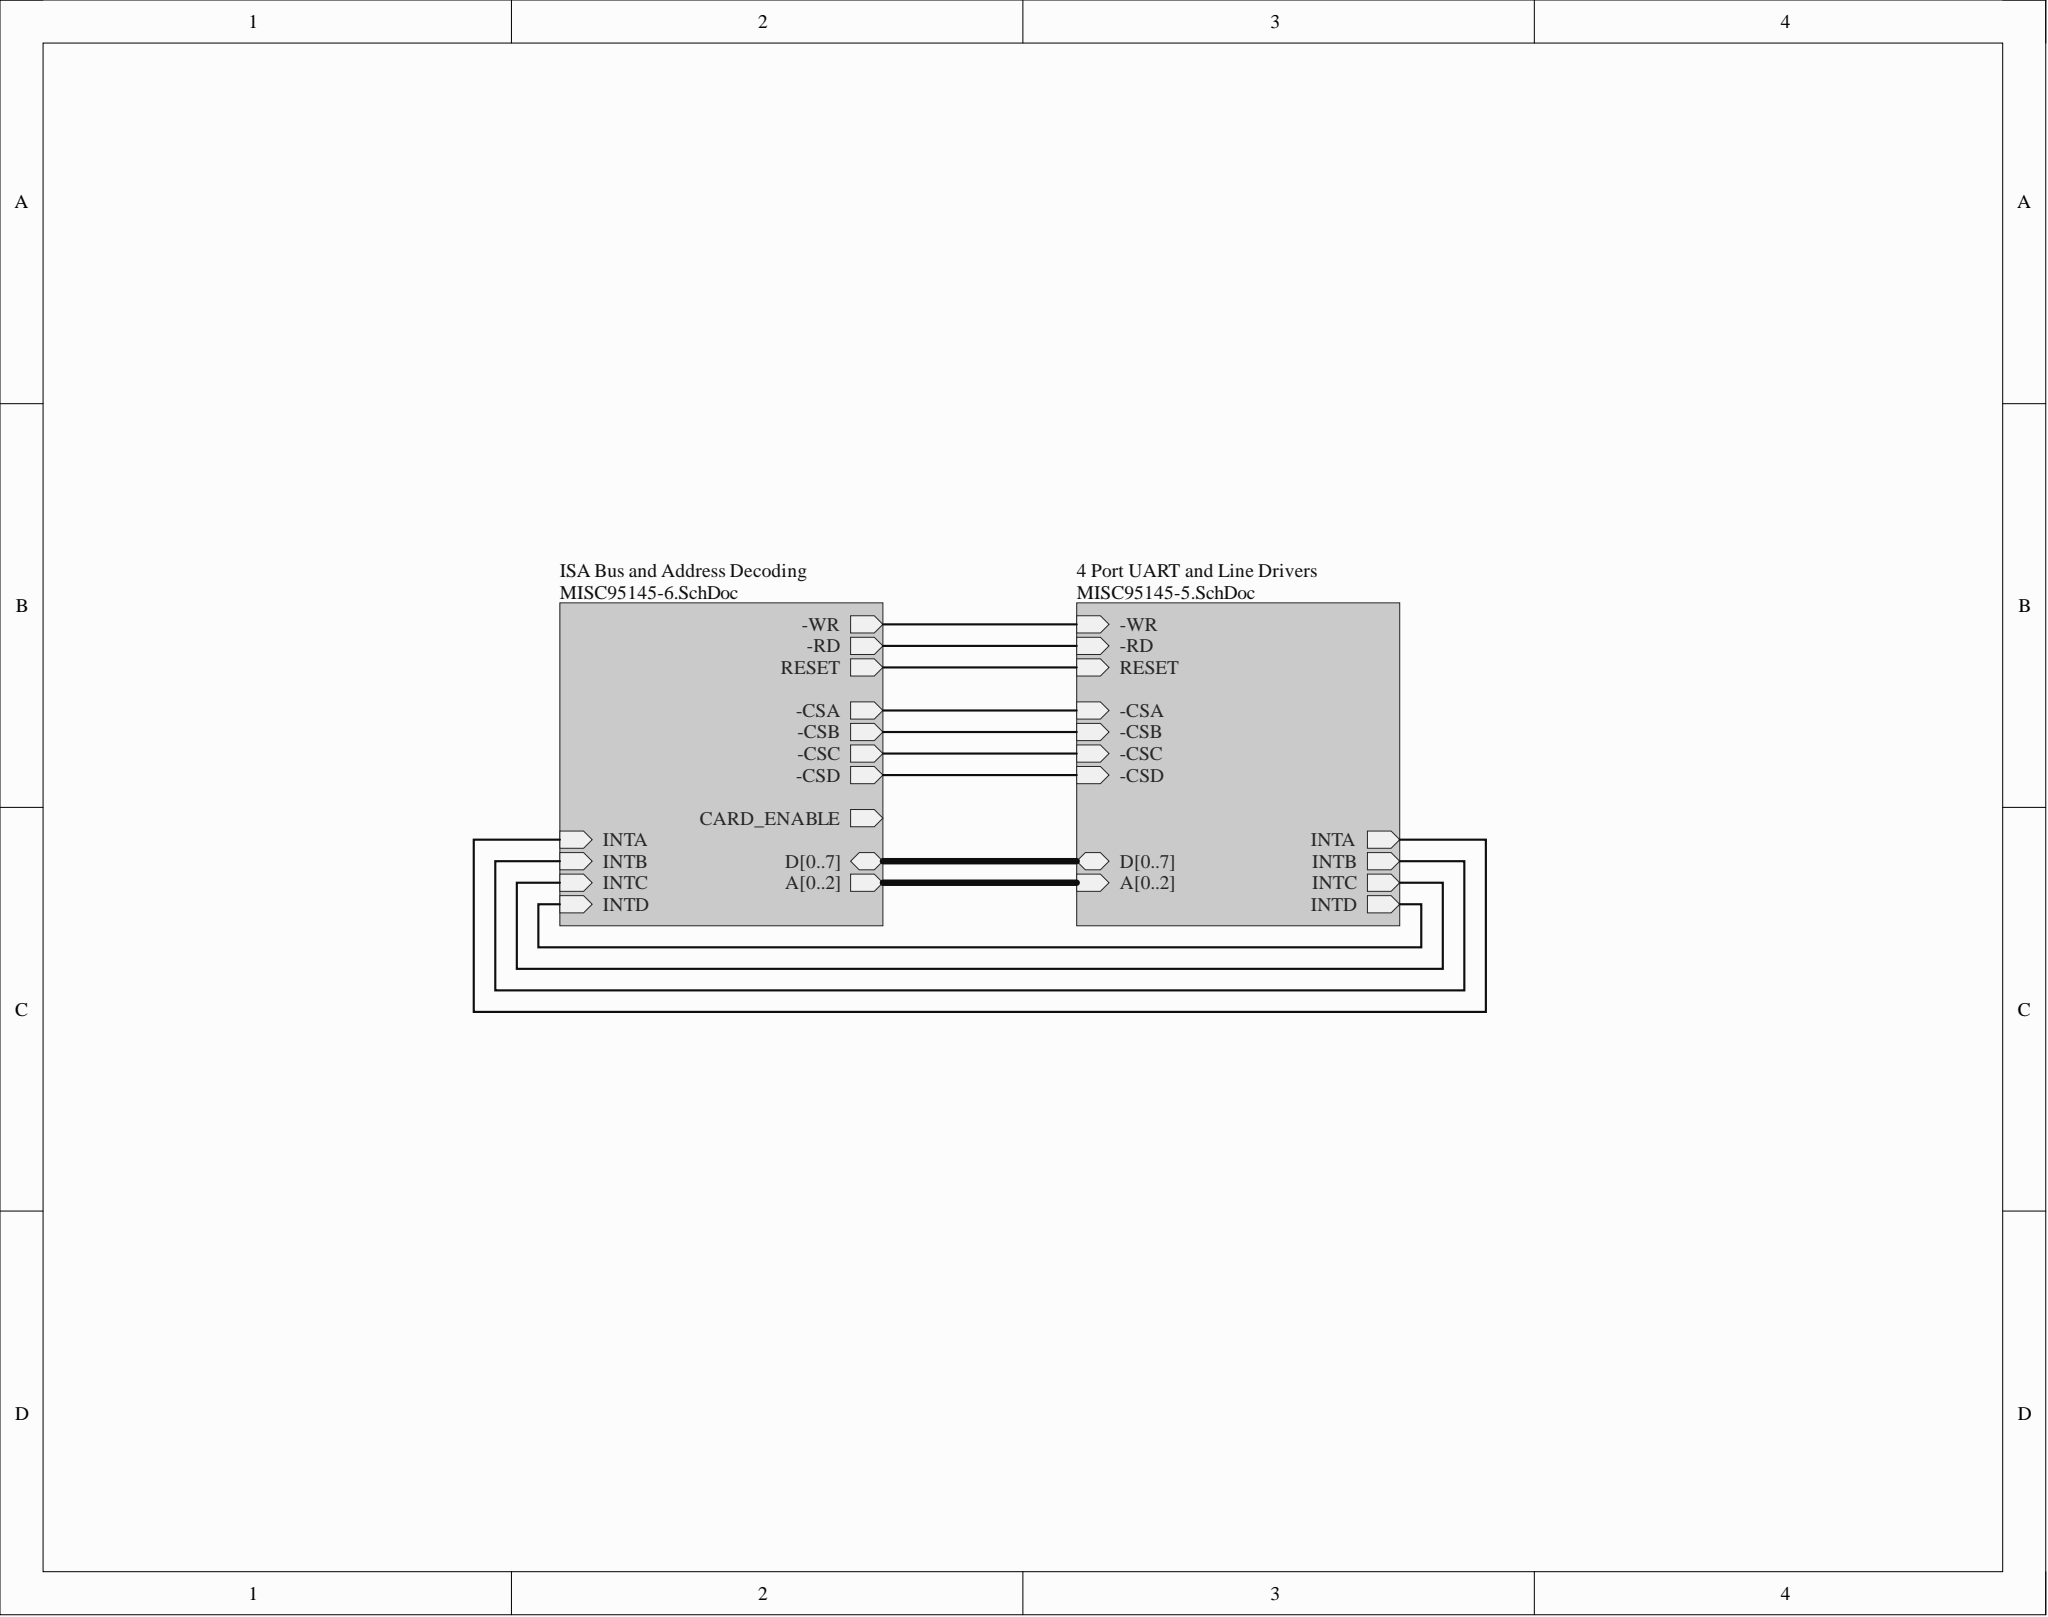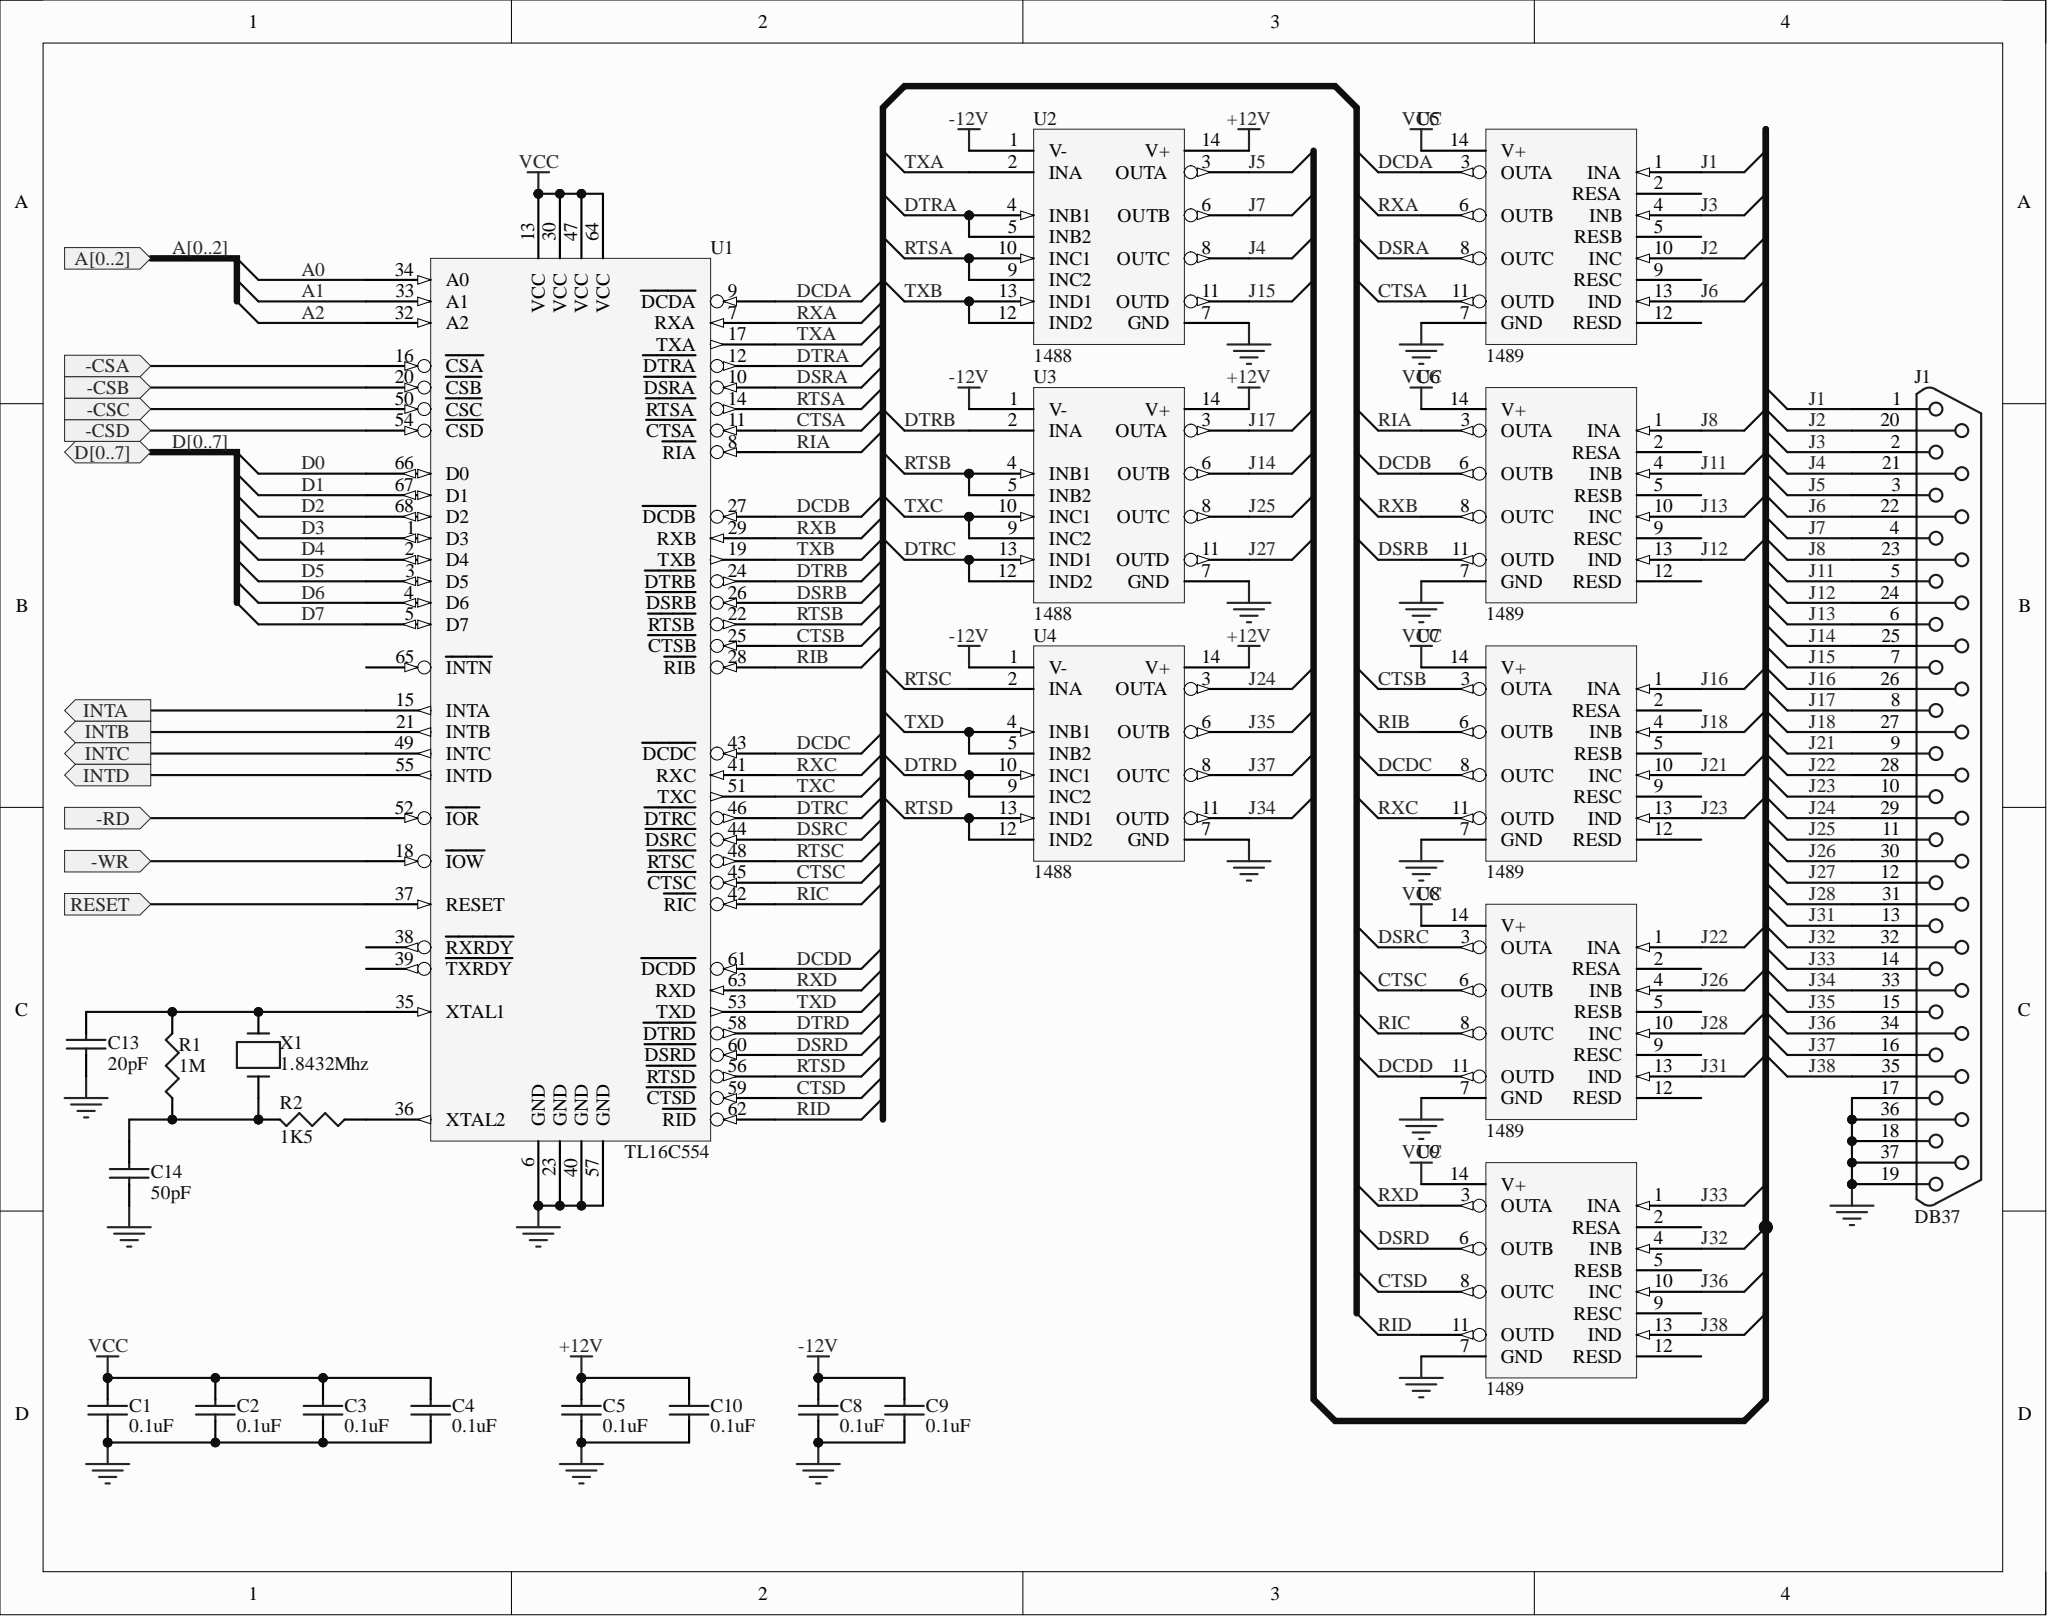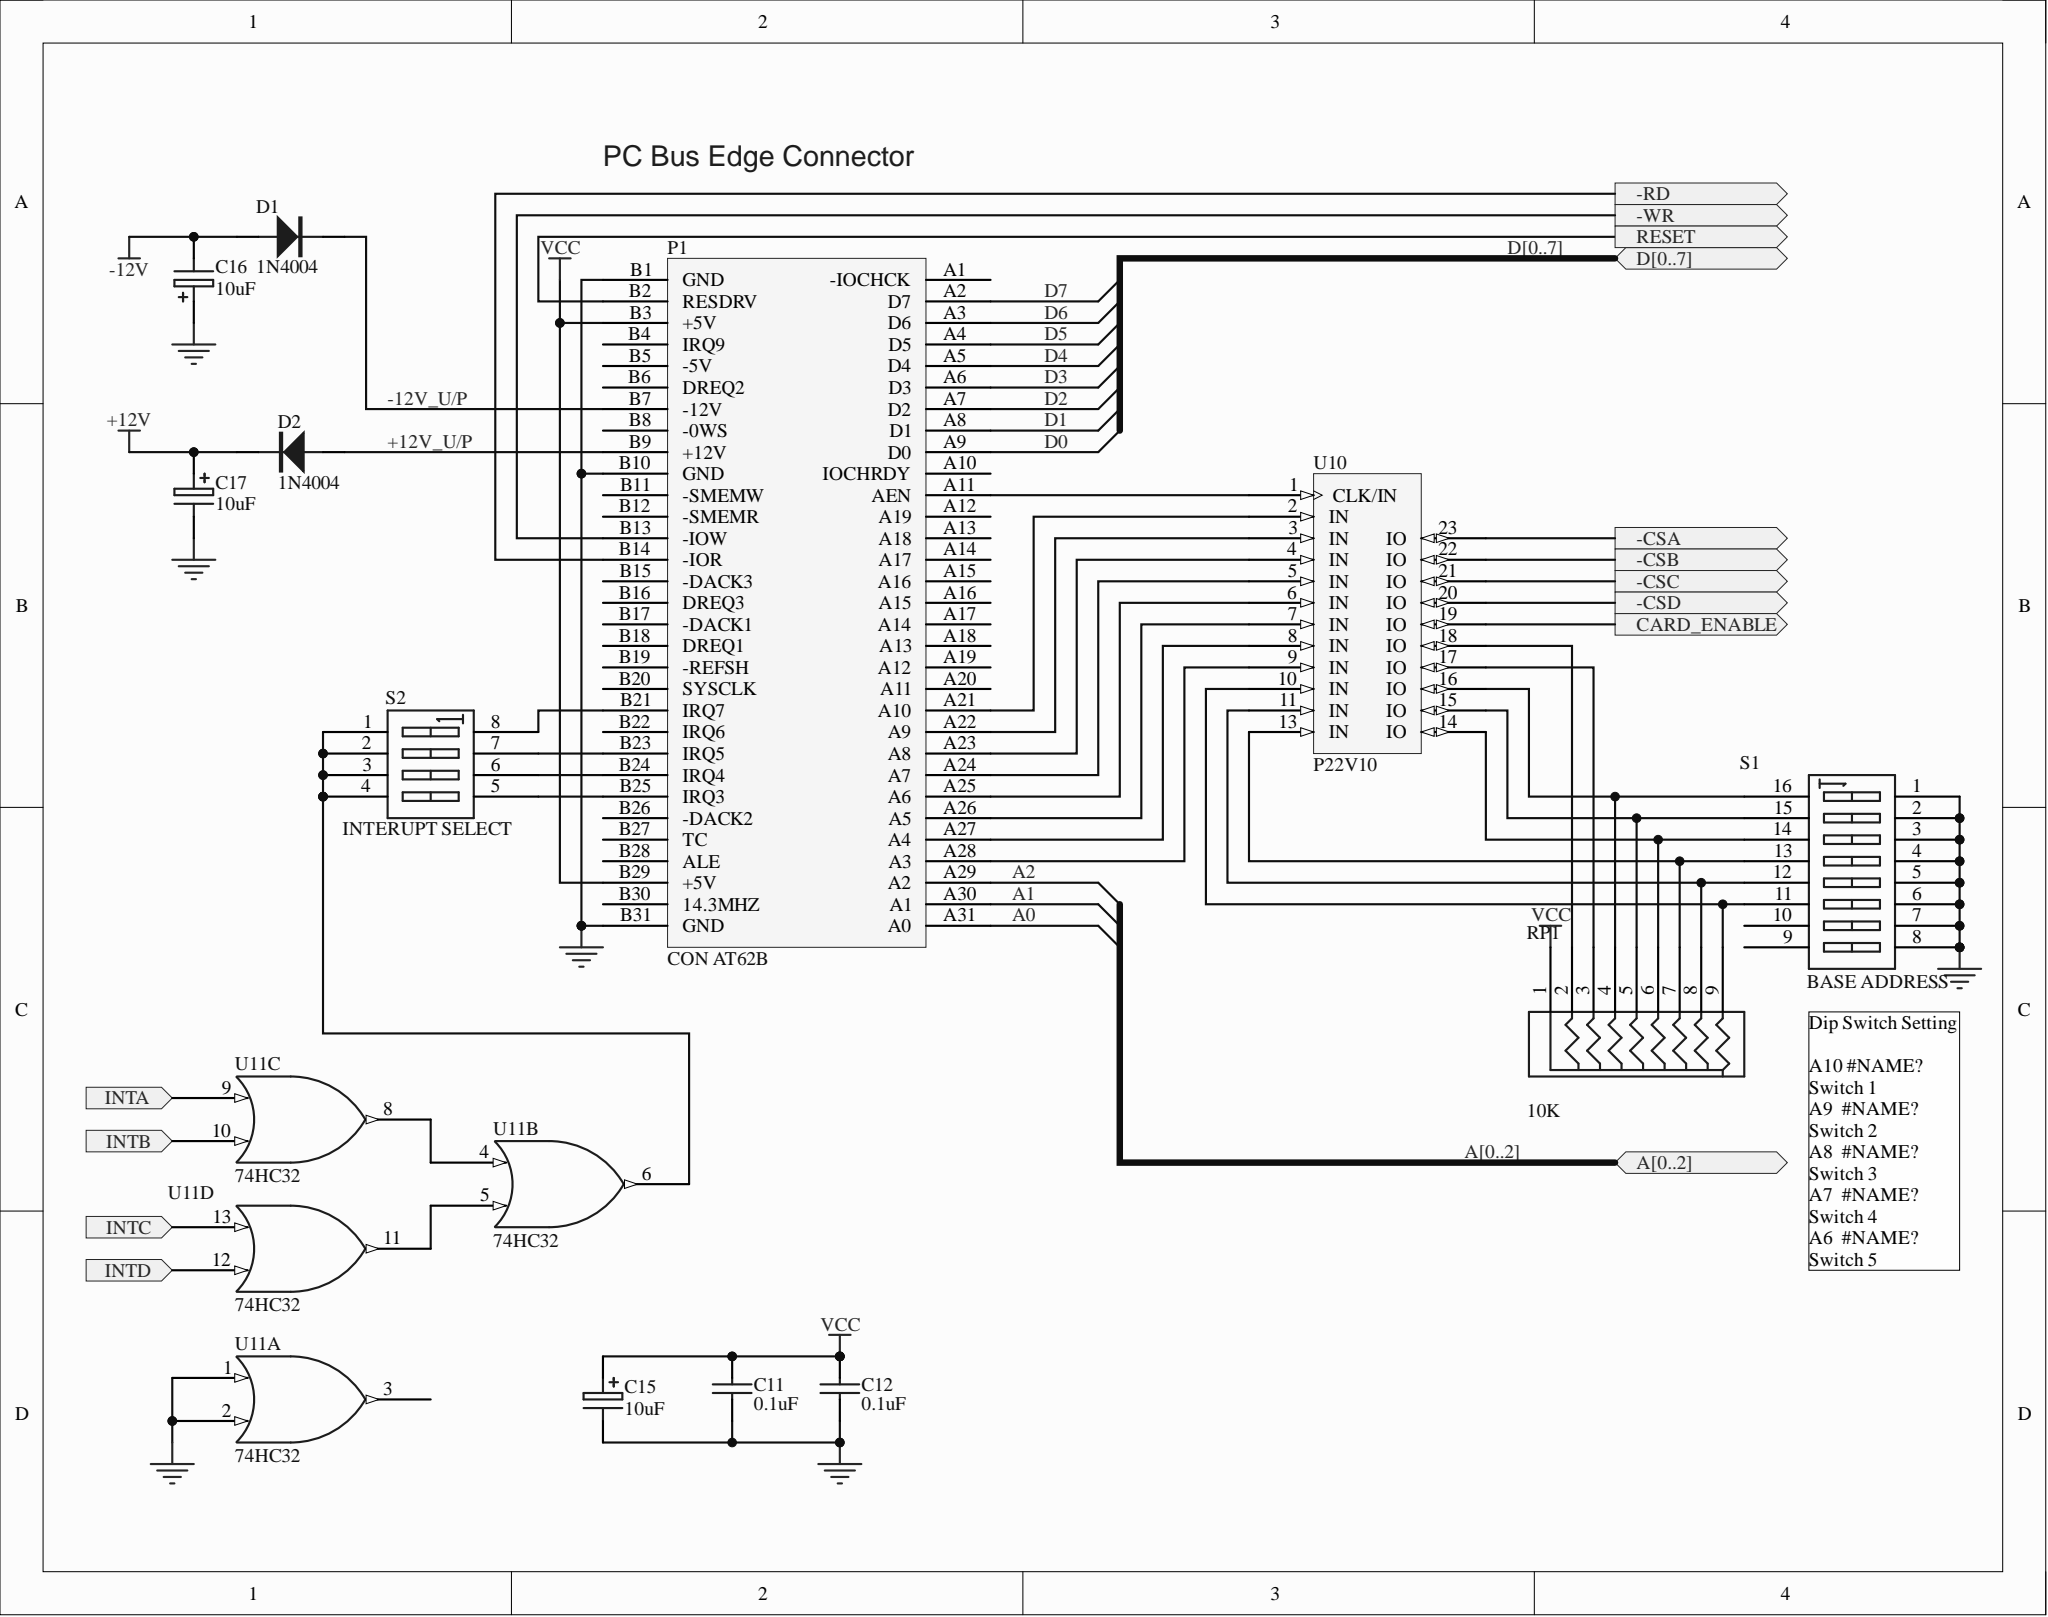Circuit board | Altium Designer | 36 parts | 119 nets
Bill of materials:
Comment,Description,Designator,Footprint,LibRef,Quantity
"0.1uF","Capacitor 0.2 pitch","C1, C2, C3, C4, C5, C8, C9, C10, C11, C12","RAD0.2","CAP 2M","10"
"20pF","Capacitor 0.2 pitch","C13","RAD0.2","CAP 2M","1"
"50pF","Capacitor 0.2 pitch","C14","RAD0.2","CAP 2M","1"
"10uF","Electrolytic Capacitor RB mount, [NoValue]","C15, C16, C17","TANT 2M/2M","ELECTRO RB, ELECTRO1","3"
"1N4004","","D1, D2","DIODE0.4","DIODE","2"
"DB37","","J1","DB37RA/F","DB37","1"
"CON AT62B","","P1","ECN-IBMXT","CON AT62B","1"
"1M","","R1","AXIAL0.4","RES1","1"
"1K5","","R2","AXIAL0.4","RES1","1"
"10K","RESISTOR NETWORK 8 COMMON RESISTORS","RP1","SIP9","RESPACK 8COMMON","1"
"BASE ADDRESS","","S1","DIP16","SW DIP-8","1"
"INTERUPT SELECT","","S2","DIP8","SW DIP-4","1"
"TL16C554","","U1","PGA68X11_SKT","TL16C554","1"
"1488","TTL-RS232 DRIVER","U2, U3, U4","DIP14","1488_1","3"
"1489","1489 RS232-TTL CONVERTOR","U5, U6, U7, U8, U9","DIP14","1489_1","5"
"P22V10","24-PIN TTL VERSATILE PAL DEVICE","U10","SDIP24","P22V10","1"
"74HC32","Quad 2-IN Pos Or G","U11","DIP14","SN7432","1"
"1.843Mhz","","X1","XTAL1","CRYSTAL","1"
Netlist (Protel format):
[
C1
RAD0.2
0.1uF



]
[
C2
RAD0.2
0.1uF



]
[
C3
RAD0.2
0.1uF



]
[
C4
RAD0.2
0.1uF



]
[
C5
RAD0.2
0.1uF



]
[
C8
RAD0.2
0.1uF



]
[
C9
RAD0.2
0.1uF



]
[
C10
RAD0.2
0.1uF



]
[
C11
RAD0.2
0.1uF



]
[
C12
RAD0.2
0.1uF



]
[
C13
RAD0.2
20pF



]
[
C14
RAD0.2
50pF



]
[
C15
TANT 2M/2M
10uF



]
[
C16
TANT 2M/2M
10uF



]
[
C17
TANT 2M/2M
10uF



]
[
D1
DIODE0.4
1N4004



]
[
D2
DIODE0.4
1N4004



]
[
J1
DB37RA/F
DB37



]
[
P1
ECN-IBMXT
CON AT62B



]
[
R1
AXIAL0.4
1M



]
[
R2
AXIAL0.4
1K5



]
[
RP1
SIP9
10K



]
[
S1
DIP16
BASE ADDRESS



]
[
S2
DIP8
INTERUPT SELECT



]
[
U1
PGA68X11_SKT
TL16C554



]
[
U2
DIP14
1488



]
[
U3
DIP14
1488



]
[
U4
DIP14
1488



]
[
U5
DIP14
1489



]
[
U6
DIP14
1489



]
[
U7
DIP14
1489



]
[
U8
DIP14
1489



]
[
U9
DIP14
1489



]
[
U10
SDIP24
P22V10



]
[
U11
DIP14
74HC32



]
[
X1
XTAL1
1.8432Mhz



]
(
VCC
C1-1
C2-1
C3-1
C4-1
C11-1
C12-1
C15-1
P1-B3
P1-B29
RP1-1
U1-13
U1-30
U1-47
U1-64
U5-14
U6-14
U7-14
U8-14
U9-14
U10-24
U11-14
)
(
TXD
U1-53
U4-4
U4-5
)
(
TXC
U1-51
U3-9
U3-10
)
(
TXB
U1-19
U2-12
U2-13
)
(
TXA
U1-17
U2-2
)
(
RXD
U1-63
U9-3
)
(
RXC
U1-41
U7-11
)
(
RXB
U1-29
U6-8
)
(
RXA
U1-7
U5-6
)
(
RTSD
U1-56
U4-12
U4-13
)
(
RTSC
U1-48
U4-2
)
(
RTSB
U1-22
U3-4
U3-5
)
(
RTSA
U1-14
U2-9
U2-10
)
(
RID
U1-62
U9-11
)
(
RIC
U1-42
U8-8
)
(
RIB
U1-28
U7-6
)
(
RIA
U1-8
U6-3
)
(
RESET
P1-B2
U1-37
)
(
NetU11_5
U11-5
U11-11
)
(
NetU11_4
U11-4
U11-8
)
(
NetS2_1
S2-1
S2-2
S2-3
S2-4
U11-6
)
(
NetRP1_9
RP1-9
S1-11
U10-10
)
(
NetRP1_8
RP1-8
S1-12
U10-11
)
(
NetRP1_7
RP1-7
S1-13
U10-13
)
(
NetRP1_6
RP1-6
S1-14
U10-14
)
(
NetRP1_5
RP1-5
S1-15
U10-15
)
(
NetRP1_4
RP1-4
S1-16
U10-16
)
(
NetRP1_3
RP1-3
U10-17
)
(
NetRP1_2
RP1-2
U10-18
)
(
NetR2_1
R2-1
U1-36
)
(
NetP1_B25
P1-B25
S2-5
)
(
NetP1_B24
P1-B24
S2-6
)
(
NetP1_B23
P1-B23
S2-7
)
(
NetP1_B21
P1-B21
S2-8
)
(
NetP1_A28
P1-A28
U10-9
)
(
NetP1_A27
P1-A27
U10-8
)
(
NetP1_A26
P1-A26
U10-7
)
(
NetP1_A25
P1-A25
U10-6
)
(
NetP1_A24
P1-A24
U10-5
)
(
NetP1_A23
P1-A23
U10-4
)
(
NetP1_A22
P1-A22
U10-3
)
(
NetP1_A21
P1-A21
U10-2
)
(
NetP1_A11
P1-A11
U10-1
)
(
NetC14_1
C14-1
R1-1
R2-2
X1-1
)
(
NetC13_1
C13-1
R1-2
U1-35
X1-2
)
(
J38
J1-35
U9-13
)
(
J37
J1-16
U4-8
)
(
J36
J1-34
U9-10
)
(
J35
J1-15
U4-6
)
(
J34
J1-33
U4-11
)
(
J33
J1-14
U9-1
)
(
J32
J1-32
U9-4
)
(
J31
J1-13
U8-13
)
(
J28
J1-31
U8-10
)
(
J27
J1-12
U3-11
)
(
J26
J1-30
U8-4
)
(
J25
J1-11
U3-8
)
(
J24
J1-29
U4-3
)
(
J23
J1-10
U7-13
)
(
J22
J1-28
U8-1
)
(
J21
J1-9
U7-10
)
(
J18
J1-27
U7-4
)
(
J17
J1-8
U3-3
)
(
J16
J1-26
U7-1
)
(
J15
J1-7
U2-11
)
(
J14
J1-25
U3-6
)
(
J13
J1-6
U6-10
)
(
J12
J1-24
U6-13
)
(
J11
J1-5
U6-4
)
(
J8
J1-23
U6-1
)
(
J7
J1-4
U2-6
)
(
J6
J1-22
U5-13
)
(
J5
J1-3
U2-3
)
(
J4
J1-21
U2-8
)
(
J3
J1-2
U5-4
)
(
J2
J1-20
U5-10
)
(
J1
J1-1
U5-1
)
(
INTD
U1-55
U11-12
)
(
INTC
U1-49
U11-13
)
(
INTB
U1-21
U11-10
)
(
INTA
U1-15
U11-9
)
(
GND
C1-2
C2-2
C3-2
C4-2
C5-2
C8-2
C9-2
C10-2
C11-2
C12-2
C13-2
C14-2
C15-2
C16-1
C17-2
J1-17
J1-18
J1-19
J1-36
J1-37
P1-B1
P1-B10
P1-B31
S1-1
S1-2
S1-3
S1-4
S1-5
S1-6
S1-7
S1-8
U1-6
U1-23
U1-40
U1-57
U2-7
U3-7
U4-7
U5-7
U6-7
U7-7
U8-7
U9-7
U10-12
U11-1
U11-2
U11-7
)
(
DTRD
U1-58
U4-9
U4-10
)
(
DTRC
U1-46
U3-12
U3-13
)
(
DTRB
U1-24
U3-2
)
(
DTRA
U1-12
U2-4
U2-5
)
(
DSRD
U1-60
U9-6
)
(
DSRC
U1-44
U8-3
)
(
DSRB
U1-26
U6-11
)
(
DSRA
U1-10
U5-8
)
(
DCDD
U1-61
U8-11
)
(
DCDC
U1-43
U7-8
)
(
DCDB
U1-27
U6-6
)
(
DCDA
U1-9
U5-3
)
(
D7
P1-A2
U1-5
)
(
D6
P1-A3
U1-4
)
(
D5
P1-A4
U1-3
)
(
D4
P1-A5
U1-2
)
(
D3
P1-A6
U1-1
)
(
D2
P1-A7
U1-68
)
(
D1
P1-A8
U1-67
)
(
D0
P1-A9
U1-66
)
(
CTSD
U1-59
U9-8
)
(
CTSC
U1-45
U8-6
)
(
CTSB
U1-25
U7-3
)
(
CTSA
U1-11
U5-11
)
(
A2
P1-A29
U1-32
)
(
A1
P1-A30
U1-33
)
(
A0
P1-A31
U1-34
)
(
-WR
P1-B13
U1-18
)
(
-RD
P1-B14
U1-52
)
(
-CSD
U1-54
U10-20
)
(
-CSC
U1-50
U10-21
)
(
-CSB
U1-20
U10-22
)
(
-CSA
U1-16
U10-23
)
(
-12V_U/P
D1-K
P1-B7
)
(
-12V
C8-1
C9-1
C16-2
D1-A
U2-1
U3-1
U4-1
)
(
+12V_U/P
D2-A
P1-B9
)
(
+12V
C5-1
C10-1
C17-1
D2-K
U2-14
U3-14
U4-14
)